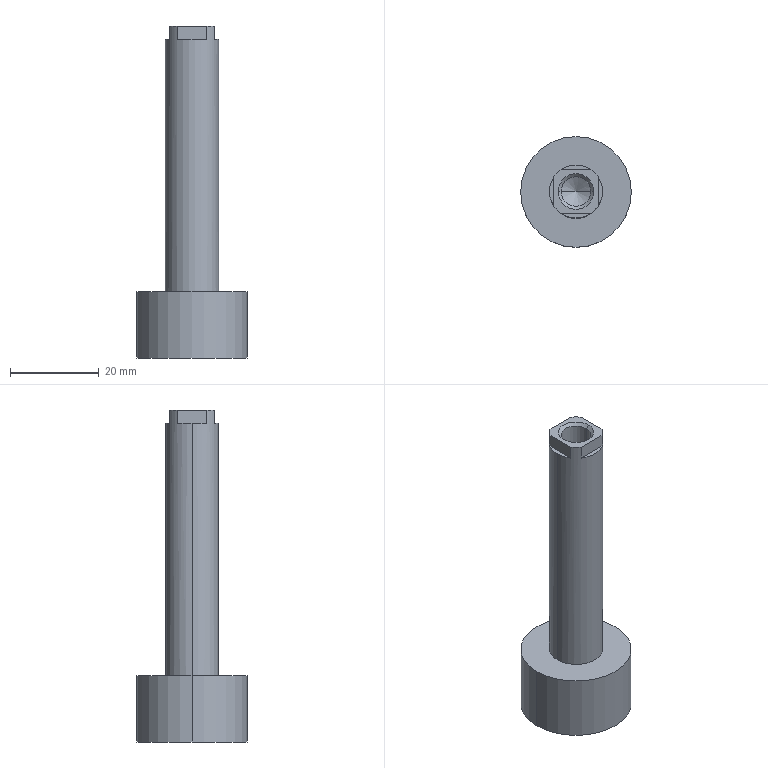Part | SolidWorks | features RefAxis 6, 3DProfileFeature 2, ICE 1, Revolution 1 | 1 solid | 21 faces | box 25 x 25 x 75 mm | volume 13686 mm3 | plane 11 | cylinder 6 | cone 4 | commonest cylinder face diameters 6.647 x2 12 x2 25 x2
STEP:
#1=CARTESIAN_POINT('',(0.,0.,7.581));
#2=VERTEX_POINT('',#1);
#3=CARTESIAN_POINT('',(3.323,0.,9.5));
#4=VERTEX_POINT('',#3);
#5=CARTESIAN_POINT('',(0.,0.,7.581));
#6=DIRECTION('',(0.866,0.,0.5));
#7=VECTOR('',#6,1000.);
#8=LINE('',#5,#7);
#9=EDGE_CURVE('',#2,#4,#8,.T.);
#10=ORIENTED_EDGE('',*,*,#9,.F.);
#11=CARTESIAN_POINT('',(-3.323,0.,9.5));
#12=VERTEX_POINT('',#11);
#13=CARTESIAN_POINT('',(0.,0.,7.581));
#14=DIRECTION('',(-0.866,0.,0.5));
#15=VECTOR('',#14,1000.);
#16=LINE('',#13,#15);
#17=EDGE_CURVE('',#2,#12,#16,.T.);
#18=ORIENTED_EDGE('',*,*,#17,.T.);
#19=CARTESIAN_POINT('',(0.,0.,9.5));
#20=DIRECTION('',(0.,0.,-1.));
#21=DIRECTION('',(-1.,0.,0.));
#22=AXIS2_PLACEMENT_3D('',#19,#20,#21);
#23=CIRCLE('',#22,3.323);
#24=EDGE_CURVE('',#4,#12,#23,.T.);
#25=ORIENTED_EDGE('',*,*,#24,.F.);
#26=EDGE_LOOP('',(#10,#18,#25));
#27=FACE_OUTER_BOUND('',#26,.T.);
#28=CARTESIAN_POINT('',(0.,0.,1007.581));
#29=DIRECTION('',(0.,0.,1.));
#30=DIRECTION('',(1.,0.,0.));
#31=AXIS2_PLACEMENT_3D('',#28,#29,#30);
#32=CONICAL_SURFACE('',#31,1732.051,1.047);
#33=ADVANCED_FACE('',(#27),#32,.F.);
#34=CARTESIAN_POINT('',(3.324,0.,19.823));
#35=VERTEX_POINT('',#34);
#36=CARTESIAN_POINT('',(-3.324,0.,19.823));
#37=VERTEX_POINT('',#36);
#38=CARTESIAN_POINT('',(0.,0.,19.823));
#39=DIRECTION('',(0.,0.,-1.));
#40=DIRECTION('',(-1.,0.,0.));
#41=AXIS2_PLACEMENT_3D('',#38,#39,#40);
#42=CIRCLE('',#41,3.324);
#43=EDGE_CURVE('',#35,#37,#42,.T.);
#44=ORIENTED_EDGE('',*,*,#43,.F.);
#45=CARTESIAN_POINT('',(3.323,0.,20.5));
#46=DIRECTION('',(0.,0.,-1.));
#47=VECTOR('',#46,1000.);
#48=LINE('',#45,#47);
#49=EDGE_CURVE('',#35,#4,#48,.T.);
#50=ORIENTED_EDGE('',*,*,#49,.T.);
#51=ORIENTED_EDGE('',*,*,#24,.T.);
#52=CARTESIAN_POINT('',(-3.323,0.,20.5));
#53=DIRECTION('',(0.,0.,-1.));
#54=VECTOR('',#53,1000.);
#55=LINE('',#52,#54);
#56=EDGE_CURVE('',#37,#12,#55,.T.);
#57=ORIENTED_EDGE('',*,*,#56,.F.);
#58=EDGE_LOOP('',(#44,#50,#51,#57));
#59=FACE_OUTER_BOUND('',#58,.T.);
#60=CARTESIAN_POINT('',(0.,0.,20.5));
#61=DIRECTION('',(0.,0.,-1.));
#62=DIRECTION('',(-1.,0.,0.));
#63=AXIS2_PLACEMENT_3D('',#60,#61,#62);
#64=CYLINDRICAL_SURFACE('',#63,3.323);
#65=ADVANCED_FACE('',(#59),#64,.F.);
#66=ORIENTED_EDGE('',*,*,#43,.T.);
#67=CARTESIAN_POINT('',(-4.,0.,20.5));
#68=VERTEX_POINT('',#67);
#69=CARTESIAN_POINT('',(-3.324,0.,19.823));
#70=DIRECTION('',(-0.7071,0.,0.7071));
#71=VECTOR('',#70,1000.);
#72=LINE('',#69,#71);
#73=EDGE_CURVE('',#37,#68,#72,.T.);
#74=ORIENTED_EDGE('',*,*,#73,.T.);
#75=CARTESIAN_POINT('',(4.,0.,20.5));
#76=VERTEX_POINT('',#75);
#77=CARTESIAN_POINT('',(0.,0.,20.5));
#78=DIRECTION('',(0.,0.,-1.));
#79=DIRECTION('',(-1.,0.,0.));
#80=AXIS2_PLACEMENT_3D('',#77,#78,#79);
#81=CIRCLE('',#80,4.);
#82=EDGE_CURVE('',#76,#68,#81,.T.);
#83=ORIENTED_EDGE('',*,*,#82,.F.);
#84=CARTESIAN_POINT('',(3.324,0.,19.823));
#85=DIRECTION('',(0.7071,0.,0.7071));
#86=VECTOR('',#85,1000.);
#87=LINE('',#84,#86);
#88=EDGE_CURVE('',#35,#76,#87,.T.);
#89=ORIENTED_EDGE('',*,*,#88,.F.);
#90=EDGE_LOOP('',(#66,#74,#83,#89));
#91=FACE_OUTER_BOUND('',#90,.T.);
#92=CARTESIAN_POINT('',(0.,0.,19.823));
#93=DIRECTION('',(0.,0.,1.));
#94=DIRECTION('',(1.,0.,0.));
#95=AXIS2_PLACEMENT_3D('',#92,#93,#94);
#96=CONICAL_SURFACE('',#95,3.324,0.7854);
#97=ADVANCED_FACE('',(#91),#96,.F.);
#98=CARTESIAN_POINT('',(-12.5,0.,-39.5));
#99=VERTEX_POINT('',#98);
#100=CARTESIAN_POINT('',(12.5,0.,-39.5));
#101=VERTEX_POINT('',#100);
#102=CARTESIAN_POINT('',(0.,0.,-39.5));
#103=DIRECTION('',(0.,0.,-1.));
#104=DIRECTION('',(-1.,0.,0.));
#105=AXIS2_PLACEMENT_3D('',#102,#103,#104);
#106=CIRCLE('',#105,12.5);
#107=EDGE_CURVE('',#99,#101,#106,.T.);
#108=ORIENTED_EDGE('',*,*,#107,.T.);
#109=CARTESIAN_POINT('',(12.5,0.,-54.5));
#110=VERTEX_POINT('',#109);
#111=CARTESIAN_POINT('',(12.5,0.,20.5));
#112=DIRECTION('',(0.,0.,-1.));
#113=VECTOR('',#112,1000.);
#114=LINE('',#111,#113);
#115=EDGE_CURVE('',#101,#110,#114,.T.);
#116=ORIENTED_EDGE('',*,*,#115,.T.);
#117=CARTESIAN_POINT('',(-12.5,0.,-54.5));
#118=VERTEX_POINT('',#117);
#119=CARTESIAN_POINT('',(0.,0.,-54.5));
#120=DIRECTION('',(0.,0.,-1.));
#121=DIRECTION('',(-1.,0.,0.));
#122=AXIS2_PLACEMENT_3D('',#119,#120,#121);
#123=CIRCLE('',#122,12.5);
#124=EDGE_CURVE('',#118,#110,#123,.T.);
#125=ORIENTED_EDGE('',*,*,#124,.F.);
#126=CARTESIAN_POINT('',(-12.5,0.,20.5));
#127=DIRECTION('',(0.,0.,-1.));
#128=VECTOR('',#127,1000.);
#129=LINE('',#126,#128);
#130=EDGE_CURVE('',#99,#118,#129,.T.);
#131=ORIENTED_EDGE('',*,*,#130,.F.);
#132=EDGE_LOOP('',(#108,#116,#125,#131));
#133=FACE_OUTER_BOUND('',#132,.T.);
#134=CARTESIAN_POINT('',(0.,0.,20.5));
#135=DIRECTION('',(0.,0.,-1.));
#136=DIRECTION('',(-1.,0.,0.));
#137=AXIS2_PLACEMENT_3D('',#134,#135,#136);
#138=CYLINDRICAL_SURFACE('',#137,12.5);
#139=ADVANCED_FACE('',(#133),#138,.T.);
#140=CARTESIAN_POINT('',(6.,0.,17.5));
#141=VERTEX_POINT('',#140);
#142=CARTESIAN_POINT('',(5.,3.317,17.5));
#143=VERTEX_POINT('',#142);
#144=CARTESIAN_POINT('',(0.,0.,17.5));
#145=DIRECTION('',(0.,0.,1.));
#146=DIRECTION('',(1.,0.,0.));
#147=AXIS2_PLACEMENT_3D('',#144,#145,#146);
#148=CIRCLE('',#147,6.);
#149=EDGE_CURVE('',#141,#143,#148,.T.);
#150=ORIENTED_EDGE('',*,*,#149,.F.);
#151=CARTESIAN_POINT('',(6.,0.,-39.5));
#152=VERTEX_POINT('',#151);
#153=CARTESIAN_POINT('',(6.,0.,20.5));
#154=DIRECTION('',(0.,0.,-1.));
#155=VECTOR('',#154,1000.);
#156=LINE('',#153,#155);
#157=EDGE_CURVE('',#141,#152,#156,.T.);
#158=ORIENTED_EDGE('',*,*,#157,.T.);
#159=CARTESIAN_POINT('',(-6.,0.,-39.5));
#160=VERTEX_POINT('',#159);
#161=CARTESIAN_POINT('',(0.,0.,-39.5));
#162=DIRECTION('',(0.,0.,-1.));
#163=DIRECTION('',(-1.,0.,0.));
#164=AXIS2_PLACEMENT_3D('',#161,#162,#163);
#165=CIRCLE('',#164,6.);
#166=EDGE_CURVE('',#160,#152,#165,.T.);
#167=ORIENTED_EDGE('',*,*,#166,.F.);
#168=CARTESIAN_POINT('',(-6.,0.,17.5));
#169=VERTEX_POINT('',#168);
#170=CARTESIAN_POINT('',(-6.,0.,20.5));
#171=DIRECTION('',(0.,0.,-1.));
#172=VECTOR('',#171,1000.);
#173=LINE('',#170,#172);
#174=EDGE_CURVE('',#169,#160,#173,.T.);
#175=ORIENTED_EDGE('',*,*,#174,.F.);
#176=CARTESIAN_POINT('',(-5.,3.317,17.5));
#177=VERTEX_POINT('',#176);
#178=CARTESIAN_POINT('',(0.,0.,17.5));
#179=DIRECTION('',(0.,0.,1.));
#180=DIRECTION('',(1.,0.,0.));
#181=AXIS2_PLACEMENT_3D('',#178,#179,#180);
#182=CIRCLE('',#181,6.);
#183=EDGE_CURVE('',#177,#169,#182,.T.);
#184=ORIENTED_EDGE('',*,*,#183,.F.);
#185=CARTESIAN_POINT('',(-5.,3.317,20.5));
#186=VERTEX_POINT('',#185);
#187=CARTESIAN_POINT('',(-5.,3.317,20.5));
#188=DIRECTION('',(0.,0.,-1.));
#189=VECTOR('',#188,1000.);
#190=LINE('',#187,#189);
#191=EDGE_CURVE('',#186,#177,#190,.T.);
#192=ORIENTED_EDGE('',*,*,#191,.F.);
#193=CARTESIAN_POINT('',(-3.317,5.,20.5));
#194=VERTEX_POINT('',#193);
#195=CARTESIAN_POINT('',(0.,0.,20.5));
#196=DIRECTION('',(0.,0.,-1.));
#197=DIRECTION('',(-1.,0.,0.));
#198=AXIS2_PLACEMENT_3D('',#195,#196,#197);
#199=CIRCLE('',#198,6.);
#200=EDGE_CURVE('',#186,#194,#199,.T.);
#201=ORIENTED_EDGE('',*,*,#200,.T.);
#202=CARTESIAN_POINT('',(-3.317,5.,17.5));
#203=VERTEX_POINT('',#202);
#204=CARTESIAN_POINT('',(-3.317,5.,20.5));
#205=DIRECTION('',(0.,0.,1.));
#206=VECTOR('',#205,1000.);
#207=LINE('',#204,#206);
#208=EDGE_CURVE('',#203,#194,#207,.T.);
#209=ORIENTED_EDGE('',*,*,#208,.F.);
#210=CARTESIAN_POINT('',(3.317,5.,17.5));
#211=VERTEX_POINT('',#210);
#212=CARTESIAN_POINT('',(0.,0.,17.5));
#213=DIRECTION('',(0.,0.,1.));
#214=DIRECTION('',(1.,0.,0.));
#215=AXIS2_PLACEMENT_3D('',#212,#213,#214);
#216=CIRCLE('',#215,6.);
#217=EDGE_CURVE('',#211,#203,#216,.T.);
#218=ORIENTED_EDGE('',*,*,#217,.F.);
#219=CARTESIAN_POINT('',(3.317,5.,20.5));
#220=VERTEX_POINT('',#219);
#221=CARTESIAN_POINT('',(3.317,5.,20.5));
#222=DIRECTION('',(0.,0.,-1.));
#223=VECTOR('',#222,1000.);
#224=LINE('',#221,#223);
#225=EDGE_CURVE('',#220,#211,#224,.T.);
#226=ORIENTED_EDGE('',*,*,#225,.F.);
#227=CARTESIAN_POINT('',(5.,3.317,20.5));
#228=VERTEX_POINT('',#227);
#229=CARTESIAN_POINT('',(0.,0.,20.5));
#230=DIRECTION('',(0.,0.,-1.));
#231=DIRECTION('',(-1.,0.,0.));
#232=AXIS2_PLACEMENT_3D('',#229,#230,#231);
#233=CIRCLE('',#232,6.);
#234=EDGE_CURVE('',#220,#228,#233,.T.);
#235=ORIENTED_EDGE('',*,*,#234,.T.);
#236=CARTESIAN_POINT('',(5.,3.317,20.5));
#237=DIRECTION('',(0.,0.,1.));
#238=VECTOR('',#237,1000.);
#239=LINE('',#236,#238);
#240=EDGE_CURVE('',#143,#228,#239,.T.);
#241=ORIENTED_EDGE('',*,*,#240,.F.);
#242=EDGE_LOOP('',(#150,#158,#167,#175,#184,#192,#201,#209,#218,#226,#235,#241));
#243=FACE_OUTER_BOUND('',#242,.T.);
#244=CARTESIAN_POINT('',(0.,0.,20.5));
#245=DIRECTION('',(0.,0.,-1.));
#246=DIRECTION('',(-1.,0.,0.));
#247=AXIS2_PLACEMENT_3D('',#244,#245,#246);
#248=CYLINDRICAL_SURFACE('',#247,6.);
#249=ADVANCED_FACE('',(#243),#248,.T.);
#250=ORIENTED_EDGE('',*,*,#157,.F.);
#251=CARTESIAN_POINT('',(5.,-3.317,17.5));
#252=VERTEX_POINT('',#251);
#253=CARTESIAN_POINT('',(0.,0.,17.5));
#254=DIRECTION('',(0.,0.,1.));
#255=DIRECTION('',(1.,0.,0.));
#256=AXIS2_PLACEMENT_3D('',#253,#254,#255);
#257=CIRCLE('',#256,6.);
#258=EDGE_CURVE('',#252,#141,#257,.T.);
#259=ORIENTED_EDGE('',*,*,#258,.F.);
#260=CARTESIAN_POINT('',(5.,-3.317,20.5));
#261=VERTEX_POINT('',#260);
#262=CARTESIAN_POINT('',(5.,-3.317,20.5));
#263=DIRECTION('',(0.,0.,-1.));
#264=VECTOR('',#263,1000.);
#265=LINE('',#262,#264);
#266=EDGE_CURVE('',#261,#252,#265,.T.);
#267=ORIENTED_EDGE('',*,*,#266,.F.);
#268=CARTESIAN_POINT('',(3.317,-5.,20.5));
#269=VERTEX_POINT('',#268);
#270=CARTESIAN_POINT('',(0.,0.,20.5));
#271=DIRECTION('',(0.,0.,-1.));
#272=DIRECTION('',(-1.,0.,0.));
#273=AXIS2_PLACEMENT_3D('',#270,#271,#272);
#274=CIRCLE('',#273,6.);
#275=EDGE_CURVE('',#261,#269,#274,.T.);
#276=ORIENTED_EDGE('',*,*,#275,.T.);
#277=CARTESIAN_POINT('',(3.317,-5.,17.5));
#278=VERTEX_POINT('',#277);
#279=CARTESIAN_POINT('',(3.317,-5.,20.5));
#280=DIRECTION('',(0.,0.,1.));
#281=VECTOR('',#280,1000.);
#282=LINE('',#279,#281);
#283=EDGE_CURVE('',#278,#269,#282,.T.);
#284=ORIENTED_EDGE('',*,*,#283,.F.);
#285=CARTESIAN_POINT('',(-3.317,-5.,17.5));
#286=VERTEX_POINT('',#285);
#287=CARTESIAN_POINT('',(0.,0.,17.5));
#288=DIRECTION('',(0.,0.,1.));
#289=DIRECTION('',(1.,0.,0.));
#290=AXIS2_PLACEMENT_3D('',#287,#288,#289);
#291=CIRCLE('',#290,6.);
#292=EDGE_CURVE('',#286,#278,#291,.T.);
#293=ORIENTED_EDGE('',*,*,#292,.F.);
#294=CARTESIAN_POINT('',(-3.317,-5.,20.5));
#295=VERTEX_POINT('',#294);
#296=CARTESIAN_POINT('',(-3.317,-5.,20.5));
#297=DIRECTION('',(0.,0.,-1.));
#298=VECTOR('',#297,1000.);
#299=LINE('',#296,#298);
#300=EDGE_CURVE('',#295,#286,#299,.T.);
#301=ORIENTED_EDGE('',*,*,#300,.F.);
#302=CARTESIAN_POINT('',(-5.,-3.317,20.5));
#303=VERTEX_POINT('',#302);
#304=CARTESIAN_POINT('',(0.,0.,20.5));
#305=DIRECTION('',(0.,0.,-1.));
#306=DIRECTION('',(-1.,0.,0.));
#307=AXIS2_PLACEMENT_3D('',#304,#305,#306);
#308=CIRCLE('',#307,6.);
#309=EDGE_CURVE('',#295,#303,#308,.T.);
#310=ORIENTED_EDGE('',*,*,#309,.T.);
#311=CARTESIAN_POINT('',(-5.,-3.317,17.5));
#312=VERTEX_POINT('',#311);
#313=CARTESIAN_POINT('',(-5.,-3.317,20.5));
#314=DIRECTION('',(0.,0.,1.));
#315=VECTOR('',#314,1000.);
#316=LINE('',#313,#315);
#317=EDGE_CURVE('',#312,#303,#316,.T.);
#318=ORIENTED_EDGE('',*,*,#317,.F.);
#319=CARTESIAN_POINT('',(0.,0.,17.5));
#320=DIRECTION('',(0.,0.,1.));
#321=DIRECTION('',(1.,0.,0.));
#322=AXIS2_PLACEMENT_3D('',#319,#320,#321);
#323=CIRCLE('',#322,6.);
#324=EDGE_CURVE('',#169,#312,#323,.T.);
#325=ORIENTED_EDGE('',*,*,#324,.F.);
#326=ORIENTED_EDGE('',*,*,#174,.T.);
#327=CARTESIAN_POINT('',(0.,0.,-39.5));
#328=DIRECTION('',(0.,0.,-1.));
#329=DIRECTION('',(-1.,0.,0.));
#330=AXIS2_PLACEMENT_3D('',#327,#328,#329);
#331=CIRCLE('',#330,6.);
#332=EDGE_CURVE('',#152,#160,#331,.T.);
#333=ORIENTED_EDGE('',*,*,#332,.F.);
#334=EDGE_LOOP('',(#250,#259,#267,#276,#284,#293,#301,#310,#318,#325,#326,#333));
#335=FACE_OUTER_BOUND('',#334,.T.);
#336=CARTESIAN_POINT('',(0.,0.,20.5));
#337=DIRECTION('',(0.,0.,-1.));
#338=DIRECTION('',(-1.,0.,0.));
#339=AXIS2_PLACEMENT_3D('',#336,#337,#338);
#340=CYLINDRICAL_SURFACE('',#339,6.);
#341=ADVANCED_FACE('',(#335),#340,.T.);
#342=ORIENTED_EDGE('',*,*,#82,.T.);
#343=CARTESIAN_POINT('',(0.,0.,20.5));
#344=DIRECTION('',(0.,0.,-1.));
#345=DIRECTION('',(-1.,0.,0.));
#346=AXIS2_PLACEMENT_3D('',#343,#344,#345);
#347=CIRCLE('',#346,4.);
#348=EDGE_CURVE('',#68,#76,#347,.T.);
#349=ORIENTED_EDGE('',*,*,#348,.T.);
#350=EDGE_LOOP('',(#342,#349));
#351=FACE_BOUND('',#350,.T.);
#352=CARTESIAN_POINT('',(6.,5.,20.5));
#353=DIRECTION('',(1.,0.,0.));
#354=VECTOR('',#353,1000.);
#355=LINE('',#352,#354);
#356=EDGE_CURVE('',#194,#220,#355,.T.);
#357=ORIENTED_EDGE('',*,*,#356,.F.);
#358=ORIENTED_EDGE('',*,*,#200,.F.);
#359=CARTESIAN_POINT('',(-5.,0.,20.5));
#360=DIRECTION('',(0.,1.,0.));
#361=VECTOR('',#360,1000.);
#362=LINE('',#359,#361);
#363=EDGE_CURVE('',#303,#186,#362,.T.);
#364=ORIENTED_EDGE('',*,*,#363,.F.);
#365=ORIENTED_EDGE('',*,*,#309,.F.);
#366=CARTESIAN_POINT('',(6.,-5.,20.5));
#367=DIRECTION('',(-1.,0.,0.));
#368=VECTOR('',#367,1000.);
#369=LINE('',#366,#368);
#370=EDGE_CURVE('',#269,#295,#369,.T.);
#371=ORIENTED_EDGE('',*,*,#370,.F.);
#372=ORIENTED_EDGE('',*,*,#275,.F.);
#373=CARTESIAN_POINT('',(5.,0.,20.5));
#374=DIRECTION('',(0.,-1.,0.));
#375=VECTOR('',#374,1000.);
#376=LINE('',#373,#375);
#377=EDGE_CURVE('',#228,#261,#376,.T.);
#378=ORIENTED_EDGE('',*,*,#377,.F.);
#379=ORIENTED_EDGE('',*,*,#234,.F.);
#380=EDGE_LOOP('',(#357,#358,#364,#365,#371,#372,#378,#379));
#381=FACE_OUTER_BOUND('',#380,.T.);
#382=CARTESIAN_POINT('',(6.,0.,20.5));
#383=DIRECTION('',(0.,0.,-1.));
#384=DIRECTION('',(-1.,0.,0.));
#385=AXIS2_PLACEMENT_3D('',#382,#383,#384);
#386=PLANE('',#385);
#387=ADVANCED_FACE('',(#351,#381),#386,.F.);
#388=ORIENTED_EDGE('',*,*,#124,.T.);
#389=CARTESIAN_POINT('',(0.,0.,-54.5));
#390=DIRECTION('',(0.,0.,-1.));
#391=DIRECTION('',(-1.,0.,0.));
#392=AXIS2_PLACEMENT_3D('',#389,#390,#391);
#393=CIRCLE('',#392,12.5);
#394=EDGE_CURVE('',#110,#118,#393,.T.);
#395=ORIENTED_EDGE('',*,*,#394,.T.);
#396=EDGE_LOOP('',(#388,#395));
#397=FACE_OUTER_BOUND('',#396,.T.);
#398=CARTESIAN_POINT('',(0.,0.,-54.5));
#399=DIRECTION('',(0.,0.,1.));
#400=DIRECTION('',(1.,0.,0.));
#401=AXIS2_PLACEMENT_3D('',#398,#399,#400);
#402=PLANE('',#401);
#403=ADVANCED_FACE('',(#397),#402,.F.);
#404=ORIENTED_EDGE('',*,*,#115,.F.);
#405=CARTESIAN_POINT('',(0.,0.,-39.5));
#406=DIRECTION('',(0.,0.,-1.));
#407=DIRECTION('',(-1.,0.,0.));
#408=AXIS2_PLACEMENT_3D('',#405,#406,#407);
#409=CIRCLE('',#408,12.5);
#410=EDGE_CURVE('',#101,#99,#409,.T.);
#411=ORIENTED_EDGE('',*,*,#410,.T.);
#412=ORIENTED_EDGE('',*,*,#130,.T.);
#413=ORIENTED_EDGE('',*,*,#394,.F.);
#414=EDGE_LOOP('',(#404,#411,#412,#413));
#415=FACE_OUTER_BOUND('',#414,.T.);
#416=CARTESIAN_POINT('',(0.,0.,20.5));
#417=DIRECTION('',(0.,0.,-1.));
#418=DIRECTION('',(-1.,0.,0.));
#419=AXIS2_PLACEMENT_3D('',#416,#417,#418);
#420=CYLINDRICAL_SURFACE('',#419,12.5);
#421=ADVANCED_FACE('',(#415),#420,.T.);
#422=ORIENTED_EDGE('',*,*,#107,.F.);
#423=ORIENTED_EDGE('',*,*,#410,.F.);
#424=EDGE_LOOP('',(#422,#423));
#425=FACE_OUTER_BOUND('',#424,.T.);
#426=ORIENTED_EDGE('',*,*,#166,.T.);
#427=ORIENTED_EDGE('',*,*,#332,.T.);
#428=EDGE_LOOP('',(#426,#427));
#429=FACE_BOUND('',#428,.T.);
#430=CARTESIAN_POINT('',(12.5,0.,-39.5));
#431=DIRECTION('',(0.,0.,-1.));
#432=DIRECTION('',(-1.,0.,0.));
#433=AXIS2_PLACEMENT_3D('',#430,#431,#432);
#434=PLANE('',#433);
#435=ADVANCED_FACE('',(#425,#429),#434,.F.);
#436=ORIENTED_EDGE('',*,*,#73,.F.);
#437=CARTESIAN_POINT('',(0.,0.,19.823));
#438=DIRECTION('',(0.,0.,-1.));
#439=DIRECTION('',(-1.,0.,0.));
#440=AXIS2_PLACEMENT_3D('',#437,#438,#439);
#441=CIRCLE('',#440,3.324);
#442=EDGE_CURVE('',#37,#35,#441,.T.);
#443=ORIENTED_EDGE('',*,*,#442,.T.);
#444=ORIENTED_EDGE('',*,*,#88,.T.);
#445=ORIENTED_EDGE('',*,*,#348,.F.);
#446=EDGE_LOOP('',(#436,#443,#444,#445));
#447=FACE_OUTER_BOUND('',#446,.T.);
#448=CARTESIAN_POINT('',(0.,0.,19.823));
#449=DIRECTION('',(0.,0.,1.));
#450=DIRECTION('',(1.,0.,0.));
#451=AXIS2_PLACEMENT_3D('',#448,#449,#450);
#452=CONICAL_SURFACE('',#451,3.324,0.7854);
#453=ADVANCED_FACE('',(#447),#452,.F.);
#454=ORIENTED_EDGE('',*,*,#49,.F.);
#455=ORIENTED_EDGE('',*,*,#442,.F.);
#456=ORIENTED_EDGE('',*,*,#56,.T.);
#457=CARTESIAN_POINT('',(0.,0.,9.5));
#458=DIRECTION('',(0.,0.,-1.));
#459=DIRECTION('',(-1.,0.,0.));
#460=AXIS2_PLACEMENT_3D('',#457,#458,#459);
#461=CIRCLE('',#460,3.323);
#462=EDGE_CURVE('',#12,#4,#461,.T.);
#463=ORIENTED_EDGE('',*,*,#462,.T.);
#464=EDGE_LOOP('',(#454,#455,#456,#463));
#465=FACE_OUTER_BOUND('',#464,.T.);
#466=CARTESIAN_POINT('',(0.,0.,20.5));
#467=DIRECTION('',(0.,0.,-1.));
#468=DIRECTION('',(-1.,0.,0.));
#469=AXIS2_PLACEMENT_3D('',#466,#467,#468);
#470=CYLINDRICAL_SURFACE('',#469,3.323);
#471=ADVANCED_FACE('',(#465),#470,.F.);
#472=ORIENTED_EDGE('',*,*,#17,.F.);
#473=ORIENTED_EDGE('',*,*,#9,.T.);
#474=ORIENTED_EDGE('',*,*,#462,.F.);
#475=EDGE_LOOP('',(#472,#473,#474));
#476=FACE_OUTER_BOUND('',#475,.T.);
#477=CARTESIAN_POINT('',(0.,0.,1007.581));
#478=DIRECTION('',(0.,0.,1.));
#479=DIRECTION('',(1.,0.,0.));
#480=AXIS2_PLACEMENT_3D('',#477,#478,#479);
#481=CONICAL_SURFACE('',#480,1732.051,1.047);
#482=ADVANCED_FACE('',(#476),#481,.F.);
#483=ORIENTED_EDGE('',*,*,#191,.T.);
#484=CARTESIAN_POINT('',(-5.,5.,17.5));
#485=DIRECTION('',(0.,-1.,0.));
#486=VECTOR('',#485,1000.);
#487=LINE('',#484,#486);
#488=EDGE_CURVE('',#177,#312,#487,.T.);
#489=ORIENTED_EDGE('',*,*,#488,.T.);
#490=ORIENTED_EDGE('',*,*,#317,.T.);
#491=ORIENTED_EDGE('',*,*,#363,.T.);
#492=EDGE_LOOP('',(#483,#489,#490,#491));
#493=FACE_OUTER_BOUND('',#492,.T.);
#494=CARTESIAN_POINT('',(-5.,5.,17.5));
#495=DIRECTION('',(-1.,0.,0.));
#496=DIRECTION('',(0.,0.,1.));
#497=AXIS2_PLACEMENT_3D('',#494,#495,#496);
#498=PLANE('',#497);
#499=ADVANCED_FACE('',(#493),#498,.T.);
#500=ORIENTED_EDGE('',*,*,#183,.T.);
#501=ORIENTED_EDGE('',*,*,#324,.T.);
#502=ORIENTED_EDGE('',*,*,#488,.F.);
#503=EDGE_LOOP('',(#500,#501,#502));
#504=FACE_OUTER_BOUND('',#503,.T.);
#505=CARTESIAN_POINT('',(0.,0.,17.5));
#506=DIRECTION('',(0.,0.,1.));
#507=DIRECTION('',(1.,0.,0.));
#508=AXIS2_PLACEMENT_3D('',#505,#506,#507);
#509=PLANE('',#508);
#510=ADVANCED_FACE('',(#504),#509,.T.);
#511=ORIENTED_EDGE('',*,*,#300,.T.);
#512=CARTESIAN_POINT('',(-5.,-5.,17.5));
#513=DIRECTION('',(1.,0.,0.));
#514=VECTOR('',#513,1000.);
#515=LINE('',#512,#514);
#516=EDGE_CURVE('',#286,#278,#515,.T.);
#517=ORIENTED_EDGE('',*,*,#516,.T.);
#518=ORIENTED_EDGE('',*,*,#283,.T.);
#519=ORIENTED_EDGE('',*,*,#370,.T.);
#520=EDGE_LOOP('',(#511,#517,#518,#519));
#521=FACE_OUTER_BOUND('',#520,.T.);
#522=CARTESIAN_POINT('',(-5.,-5.,17.5));
#523=DIRECTION('',(0.,-1.,0.));
#524=DIRECTION('',(0.,0.,-1.));
#525=AXIS2_PLACEMENT_3D('',#522,#523,#524);
#526=PLANE('',#525);
#527=ADVANCED_FACE('',(#521),#526,.T.);
#528=ORIENTED_EDGE('',*,*,#292,.T.);
#529=ORIENTED_EDGE('',*,*,#516,.F.);
#530=EDGE_LOOP('',(#528,#529));
#531=FACE_OUTER_BOUND('',#530,.T.);
#532=CARTESIAN_POINT('',(0.,0.,17.5));
#533=DIRECTION('',(0.,0.,1.));
#534=DIRECTION('',(1.,0.,0.));
#535=AXIS2_PLACEMENT_3D('',#532,#533,#534);
#536=PLANE('',#535);
#537=ADVANCED_FACE('',(#531),#536,.T.);
#538=ORIENTED_EDGE('',*,*,#266,.T.);
#539=CARTESIAN_POINT('',(5.,-5.,17.5));
#540=DIRECTION('',(0.,1.,0.));
#541=VECTOR('',#540,1000.);
#542=LINE('',#539,#541);
#543=EDGE_CURVE('',#252,#143,#542,.T.);
#544=ORIENTED_EDGE('',*,*,#543,.T.);
#545=ORIENTED_EDGE('',*,*,#240,.T.);
#546=ORIENTED_EDGE('',*,*,#377,.T.);
#547=EDGE_LOOP('',(#538,#544,#545,#546));
#548=FACE_OUTER_BOUND('',#547,.T.);
#549=CARTESIAN_POINT('',(5.,-5.,17.5));
#550=DIRECTION('',(1.,0.,0.));
#551=DIRECTION('',(0.,0.,-1.));
#552=AXIS2_PLACEMENT_3D('',#549,#550,#551);
#553=PLANE('',#552);
#554=ADVANCED_FACE('',(#548),#553,.T.);
#555=ORIENTED_EDGE('',*,*,#258,.T.);
#556=ORIENTED_EDGE('',*,*,#149,.T.);
#557=ORIENTED_EDGE('',*,*,#543,.F.);
#558=EDGE_LOOP('',(#555,#556,#557));
#559=FACE_OUTER_BOUND('',#558,.T.);
#560=CARTESIAN_POINT('',(0.,0.,17.5));
#561=DIRECTION('',(0.,0.,1.));
#562=DIRECTION('',(1.,0.,0.));
#563=AXIS2_PLACEMENT_3D('',#560,#561,#562);
#564=PLANE('',#563);
#565=ADVANCED_FACE('',(#559),#564,.T.);
#566=ORIENTED_EDGE('',*,*,#217,.T.);
#567=CARTESIAN_POINT('',(5.,5.,17.5));
#568=DIRECTION('',(-1.,0.,0.));
#569=VECTOR('',#568,1000.);
#570=LINE('',#567,#569);
#571=EDGE_CURVE('',#211,#203,#570,.T.);
#572=ORIENTED_EDGE('',*,*,#571,.F.);
#573=EDGE_LOOP('',(#566,#572));
#574=FACE_OUTER_BOUND('',#573,.T.);
#575=CARTESIAN_POINT('',(0.,0.,17.5));
#576=DIRECTION('',(0.,0.,1.));
#577=DIRECTION('',(1.,0.,0.));
#578=AXIS2_PLACEMENT_3D('',#575,#576,#577);
#579=PLANE('',#578);
#580=ADVANCED_FACE('',(#574),#579,.T.);
#581=ORIENTED_EDGE('',*,*,#225,.T.);
#582=ORIENTED_EDGE('',*,*,#571,.T.);
#583=ORIENTED_EDGE('',*,*,#208,.T.);
#584=ORIENTED_EDGE('',*,*,#356,.T.);
#585=EDGE_LOOP('',(#581,#582,#583,#584));
#586=FACE_OUTER_BOUND('',#585,.T.);
#587=CARTESIAN_POINT('',(5.,5.,17.5));
#588=DIRECTION('',(0.,1.,0.));
#589=DIRECTION('',(0.,0.,1.));
#590=AXIS2_PLACEMENT_3D('',#587,#588,#589);
#591=PLANE('',#590);
#592=ADVANCED_FACE('',(#586),#591,.T.);
#593=CLOSED_SHELL('',(#33,#65,#97,#139,#249,#341,#387,#403,#421,#435,#453,#471,#482,#499,#510,#527,#537,#554,#565,#580,#592));
#594=MANIFOLD_SOLID_BREP('',#593);
#595=CARTESIAN_POINT('',(0.,0.,0.));
#596=DIRECTION('',(0.,0.,1.));
#597=DIRECTION('',(1.,0.,0.));
#598=AXIS2_PLACEMENT_3D('',#595,#596,#597);
#599=(LENGTH_UNIT()NAMED_UNIT(*)SI_UNIT(.MILLI.,.METRE.));
#600=UNCERTAINTY_MEASURE_WITH_UNIT(LENGTH_MEASURE(0.00001),#599,'','');
#601=(NAMED_UNIT(*)PLANE_ANGLE_UNIT()SI_UNIT($,.RADIAN.));
#602=(NAMED_UNIT(*)SI_UNIT($,.STERADIAN.)SOLID_ANGLE_UNIT());
#603=(GEOMETRIC_REPRESENTATION_CONTEXT(3)GLOBAL_UNCERTAINTY_ASSIGNED_CONTEXT((#600))GLOBAL_UNIT_ASSIGNED_CONTEXT((#599,#601,#602))REPRESENTATION_CONTEXT('',''));
#604=ADVANCED_BREP_SHAPE_REPRESENTATION('',(#594,#598),#603);